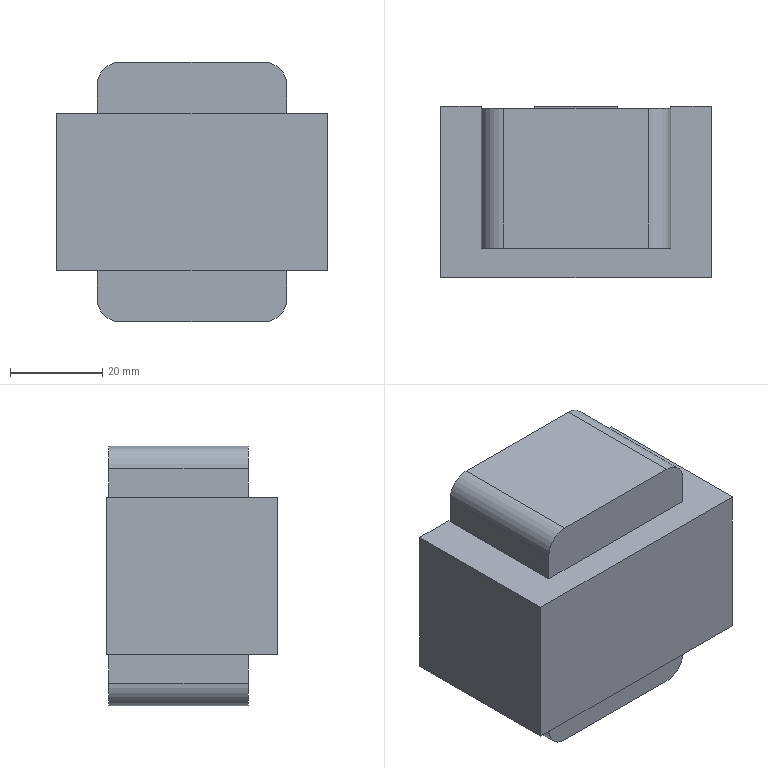Part | STEP file | 1 solid | 27 faces | box 58.8 x 37.24 x 56.35 mm | volume 101666 mm3 | plane 23 | cylinder 4 | commonest cylinder face diameters 9.8 x4